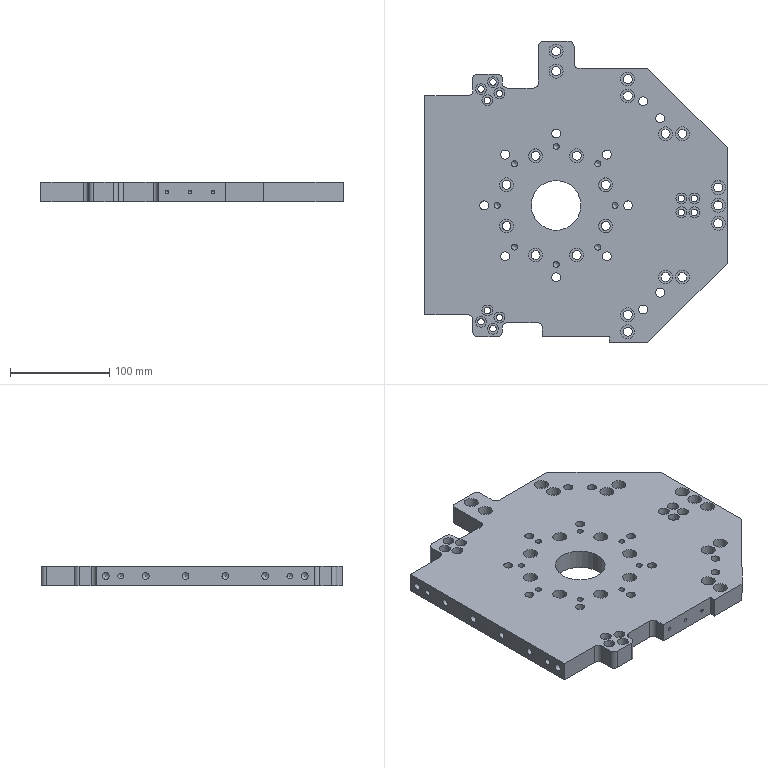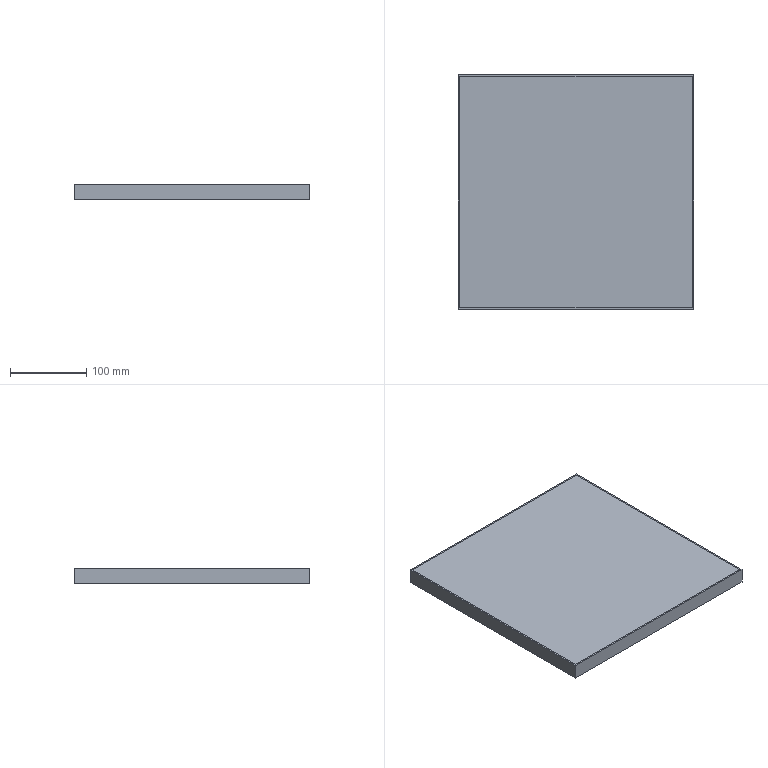CAM job | NX | 3-axis milling, drilling | part box 304 x 303 x 20 mm | stock box 308 x 307 x 20 mm
Tools:
number,name,description,diameter,corner_radius,flute_length,length,flutes
11,ZXZ,Milling Tool-5 Parameters,6.0,0.0,50.0,75.0,2
16,6.0ZT,Drilling Tool,6.0,0.0,35.0,50.0,2
19,9.0ZT,Drilling Tool,9.0,0.0,35.0,50.0,2
17,6.6ZT,Drilling Tool,6.6,0.0,35.0,50.0,2
10,D10,Milling Tool-5 Parameters,10.0,0.0,50.0,75.0,2
6,D6,Milling Tool-5 Parameters,6.0,0.0,50.0,75.0,2
9,D10JING,Milling Tool-5 Parameters,10.0,0.0,50.0,75.0,2
7,D6A45,Milling Tool-5 Parameters,6.0,0.0,3.0,3.0,2
Operations:
program,operation,operation_type,tool,method,geometry_group,spindle_rpm,surface_speed,feed_per_tooth,feed_cut,feed_plunge,cut_length_mm,path_length_mm,cut_time_min,machine_time_min
1压左右,DRILLING,Operation,ZXZ,METHOD,A,3000.0,56.0,0.0417,250.0,0.0,216.0,2114.027,0.864,1.054
1压左右,DRILLING_COPY,Operation,6.0ZT,METHOD,A,2000.0,37.0,0.045,180.0,0.0,158.421,815.971,0.8801,0.9459
1压左右,DRILLING_COPY_COPY,Operation,9.0ZT,METHOD,A,1000.0,28.0,0.09,180.0,0.0,881.228,2994.526,4.896,5.107
1压左右,DRILLING_COPY_COPY_COPY,Operation,9.0ZT,METHOD,A,1000.0,28.0,0.09,180.0,0.0,26.704,213.408,0.1484,0.167
1压左右,DRILLING_COPY_COPY_1,Operation,6.6ZT,METHOD,A,2000.0,37.0,0.045,180.0,0.0,311.794,1362.111,1.732,1.837
1压左右,HOLE_MILLING,CylinderMilling,D10,METHOD,A,3200.0,100.0,0.3438,2200.0,100.0,14078.145,18512.076,6.399,6.843
1压左右,HOLE_MILLING_COPY_1,CylinderMilling,D10,METHOD,A,3200.0,100.0,0.3438,2200.0,100.0,7456.676,7636.176,3.389,3.407
1压左右,ZLEVEL_PROFILE,ZLevelMilling,D10,METHOD,A,2200.0,69.0,0.5,2200.0,100.0,35621.693,36337.39,16.192,16.263
1压左右,HOLE_MILLING_COPY,CylinderMilling,D6,METHOD,A,4000.0,75.0,0.2062,1650.0,100.0,14420.197,16961.674,8.739,8.994
1压左右,ZLEVEL_PROFILE_COPY,ZLevelMilling,D10JING,METHOD,A,5000.0,157.0,0.12,1200.0,100.0,370.596,1085.726,0.3088,0.3803
1压左右,ZLEVEL_PROFILE_COPY_COPY,ZLevelMilling,D6A45,METHOD,A,7500.0,141.0,0.08,1200.0,100.0,2551.091,19072.899,2.126,3.778
1压左右,刀补9,ZLevelMilling,D10JING,METHOD,A,5000.0,157.0,0.12,1200.0,100.0,145.133,339.133,0.1209,0.1403
2压前后,ZLEVEL_PROFILE_COPY_1,ZLevelMilling,D10,METHOD,A,2200.0,69.0,0.5,2200.0,100.0,79467.374,80094.925,36.121,36.184
2压前后,ZLEVEL_PROFILE_COPY_COPY_1,ZLevelMilling,D10JING,METHOD,A,5000.0,157.0,0.12,1200.0,100.0,852.679,1479.65,0.7106,0.7733
2压前后,ZLEVEL_PROFILE_COPY_COPY_COPY,ZLevelMilling,D6A45,METHOD,A,7500.0,141.0,0.08,1200.0,100.0,838.259,1374.082,0.6985,0.7521
2夹夹着做,HOLE_MILLING_COPY_2,CylinderMilling,D10,METHOD,B,3200.0,100.0,0.3438,2200.0,100.0,6738.857,9354.288,3.063,3.325
2夹夹着做,ZLEVEL_PROFILE_COPY_COPY_COPY_1,ZLevelMilling,D6A45,METHOD,B,7500.0,141.0,0.08,1200.0,100.0,2873.551,17731.962,2.395,3.881